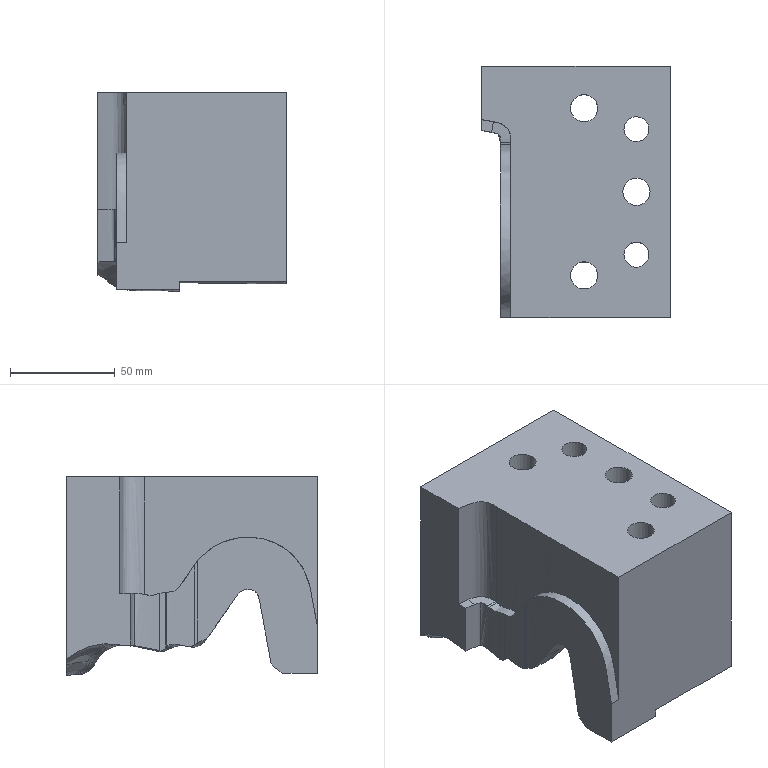Part | NX | features solid 2 | 1 solid | 72 faces | box 90 x 120 x 94.794 mm | volume 641655 mm3 | spline 47 | plane 13 | cylinder 12 | commonest cylinder face diameters 13 x3 20 x3 11.101 x2 12 x2 9 x1 14 x1